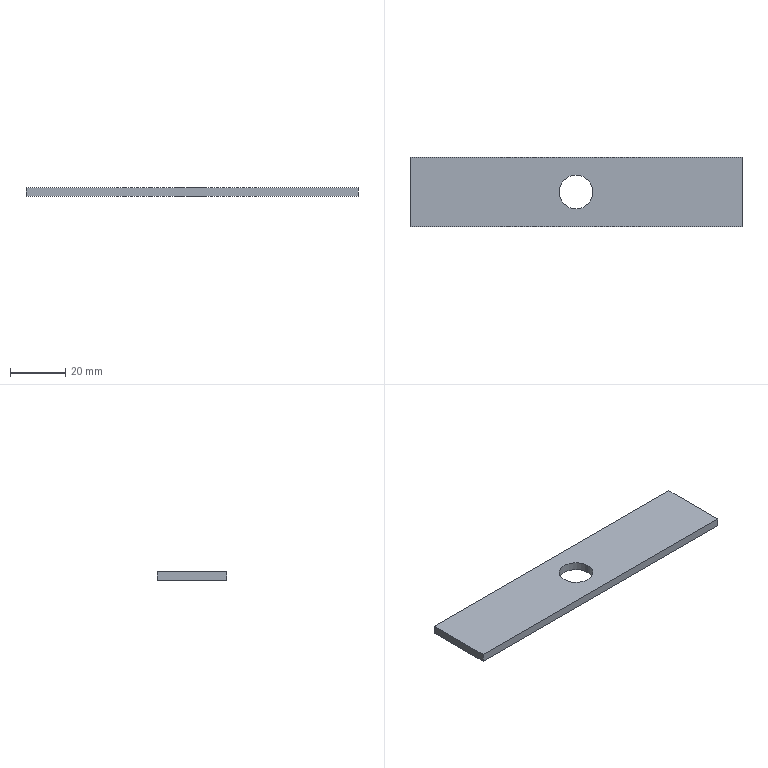Part | SolidWorks | features Extrusion 1, ICE 1 | 1 solid | 8 faces | box 120 x 25 x 3 mm | volume 8649 mm3 | plane 6 | cylinder 2 | commonest cylinder face diameters 12.2 x2
STEP:
#1=CARTESIAN_POINT('',(-6.1,0.,-1.5));
#2=VERTEX_POINT('',#1);
#3=CARTESIAN_POINT('',(6.1,0.,-1.5));
#4=VERTEX_POINT('',#3);
#5=CARTESIAN_POINT('',(0.,0.,-1.5));
#6=DIRECTION('',(0.,0.,1.));
#7=DIRECTION('',(1.,0.,0.));
#8=AXIS2_PLACEMENT_3D('',#5,#6,#7);
#9=CIRCLE('',#8,6.1);
#10=EDGE_CURVE('',#2,#4,#9,.T.);
#11=ORIENTED_EDGE('',*,*,#10,.F.);
#12=CARTESIAN_POINT('',(-6.1,0.,1.5));
#13=VERTEX_POINT('',#12);
#14=CARTESIAN_POINT('',(-6.1,0.,-11.5));
#15=DIRECTION('',(0.,0.,1.));
#16=VECTOR('',#15,1000.);
#17=LINE('',#14,#16);
#18=EDGE_CURVE('',#2,#13,#17,.T.);
#19=ORIENTED_EDGE('',*,*,#18,.T.);
#20=CARTESIAN_POINT('',(6.1,0.,1.5));
#21=VERTEX_POINT('',#20);
#22=CARTESIAN_POINT('',(0.,0.,1.5));
#23=DIRECTION('',(0.,0.,1.));
#24=DIRECTION('',(1.,0.,0.));
#25=AXIS2_PLACEMENT_3D('',#22,#23,#24);
#26=CIRCLE('',#25,6.1);
#27=EDGE_CURVE('',#13,#21,#26,.T.);
#28=ORIENTED_EDGE('',*,*,#27,.T.);
#29=CARTESIAN_POINT('',(6.1,0.,-11.5));
#30=DIRECTION('',(0.,0.,1.));
#31=VECTOR('',#30,1000.);
#32=LINE('',#29,#31);
#33=EDGE_CURVE('',#4,#21,#32,.T.);
#34=ORIENTED_EDGE('',*,*,#33,.F.);
#35=EDGE_LOOP('',(#11,#19,#28,#34));
#36=FACE_OUTER_BOUND('',#35,.T.);
#37=CARTESIAN_POINT('',(0.,0.,-11.5));
#38=DIRECTION('',(0.,0.,1.));
#39=DIRECTION('',(1.,0.,0.));
#40=AXIS2_PLACEMENT_3D('',#37,#38,#39);
#41=CYLINDRICAL_SURFACE('',#40,6.1);
#42=ADVANCED_FACE('',(#36),#41,.F.);
#43=CARTESIAN_POINT('',(-60.,12.5,1.5));
#44=VERTEX_POINT('',#43);
#45=CARTESIAN_POINT('',(-60.,-12.5,1.5));
#46=VERTEX_POINT('',#45);
#47=CARTESIAN_POINT('',(-60.,12.5,1.5));
#48=DIRECTION('',(0.,-1.,0.));
#49=VECTOR('',#48,1000.);
#50=LINE('',#47,#49);
#51=EDGE_CURVE('',#44,#46,#50,.T.);
#52=ORIENTED_EDGE('',*,*,#51,.F.);
#53=CARTESIAN_POINT('',(-60.,12.5,-1.5));
#54=VERTEX_POINT('',#53);
#55=CARTESIAN_POINT('',(-60.,12.5,-1.5));
#56=DIRECTION('',(0.,0.,1.));
#57=VECTOR('',#56,1000.);
#58=LINE('',#55,#57);
#59=EDGE_CURVE('',#54,#44,#58,.T.);
#60=ORIENTED_EDGE('',*,*,#59,.F.);
#61=CARTESIAN_POINT('',(-60.,-12.5,-1.5));
#62=VERTEX_POINT('',#61);
#63=CARTESIAN_POINT('',(-60.,12.5,-1.5));
#64=DIRECTION('',(0.,-1.,0.));
#65=VECTOR('',#64,1000.);
#66=LINE('',#63,#65);
#67=EDGE_CURVE('',#54,#62,#66,.T.);
#68=ORIENTED_EDGE('',*,*,#67,.T.);
#69=CARTESIAN_POINT('',(-60.,-12.5,-1.5));
#70=DIRECTION('',(0.,0.,1.));
#71=VECTOR('',#70,1000.);
#72=LINE('',#69,#71);
#73=EDGE_CURVE('',#62,#46,#72,.T.);
#74=ORIENTED_EDGE('',*,*,#73,.T.);
#75=EDGE_LOOP('',(#52,#60,#68,#74));
#76=FACE_OUTER_BOUND('',#75,.T.);
#77=CARTESIAN_POINT('',(-60.,12.5,-1.5));
#78=DIRECTION('',(-1.,0.,0.));
#79=DIRECTION('',(0.,0.,1.));
#80=AXIS2_PLACEMENT_3D('',#77,#78,#79);
#81=PLANE('',#80);
#82=ADVANCED_FACE('',(#76),#81,.T.);
#83=CARTESIAN_POINT('',(60.,12.5,1.5));
#84=VERTEX_POINT('',#83);
#85=CARTESIAN_POINT('',(60.,12.5,1.5));
#86=DIRECTION('',(-1.,0.,0.));
#87=VECTOR('',#86,1000.);
#88=LINE('',#85,#87);
#89=EDGE_CURVE('',#84,#44,#88,.T.);
#90=ORIENTED_EDGE('',*,*,#89,.F.);
#91=CARTESIAN_POINT('',(60.,12.5,-1.5));
#92=VERTEX_POINT('',#91);
#93=CARTESIAN_POINT('',(60.,12.5,-1.5));
#94=DIRECTION('',(0.,0.,1.));
#95=VECTOR('',#94,1000.);
#96=LINE('',#93,#95);
#97=EDGE_CURVE('',#92,#84,#96,.T.);
#98=ORIENTED_EDGE('',*,*,#97,.F.);
#99=CARTESIAN_POINT('',(60.,12.5,-1.5));
#100=DIRECTION('',(-1.,0.,0.));
#101=VECTOR('',#100,1000.);
#102=LINE('',#99,#101);
#103=EDGE_CURVE('',#92,#54,#102,.T.);
#104=ORIENTED_EDGE('',*,*,#103,.T.);
#105=ORIENTED_EDGE('',*,*,#59,.T.);
#106=EDGE_LOOP('',(#90,#98,#104,#105));
#107=FACE_OUTER_BOUND('',#106,.T.);
#108=CARTESIAN_POINT('',(60.,12.5,-1.5));
#109=DIRECTION('',(0.,1.,0.));
#110=DIRECTION('',(0.,0.,1.));
#111=AXIS2_PLACEMENT_3D('',#108,#109,#110);
#112=PLANE('',#111);
#113=ADVANCED_FACE('',(#107),#112,.T.);
#114=CARTESIAN_POINT('',(60.,-12.5,1.5));
#115=VERTEX_POINT('',#114);
#116=CARTESIAN_POINT('',(60.,-12.5,1.5));
#117=DIRECTION('',(0.,1.,0.));
#118=VECTOR('',#117,1000.);
#119=LINE('',#116,#118);
#120=EDGE_CURVE('',#115,#84,#119,.T.);
#121=ORIENTED_EDGE('',*,*,#120,.F.);
#122=CARTESIAN_POINT('',(60.,-12.5,-1.5));
#123=VERTEX_POINT('',#122);
#124=CARTESIAN_POINT('',(60.,-12.5,-1.5));
#125=DIRECTION('',(0.,0.,1.));
#126=VECTOR('',#125,1000.);
#127=LINE('',#124,#126);
#128=EDGE_CURVE('',#123,#115,#127,.T.);
#129=ORIENTED_EDGE('',*,*,#128,.F.);
#130=CARTESIAN_POINT('',(60.,-12.5,-1.5));
#131=DIRECTION('',(0.,1.,0.));
#132=VECTOR('',#131,1000.);
#133=LINE('',#130,#132);
#134=EDGE_CURVE('',#123,#92,#133,.T.);
#135=ORIENTED_EDGE('',*,*,#134,.T.);
#136=ORIENTED_EDGE('',*,*,#97,.T.);
#137=EDGE_LOOP('',(#121,#129,#135,#136));
#138=FACE_OUTER_BOUND('',#137,.T.);
#139=CARTESIAN_POINT('',(60.,-12.5,-1.5));
#140=DIRECTION('',(1.,0.,0.));
#141=DIRECTION('',(0.,0.,-1.));
#142=AXIS2_PLACEMENT_3D('',#139,#140,#141);
#143=PLANE('',#142);
#144=ADVANCED_FACE('',(#138),#143,.T.);
#145=CARTESIAN_POINT('',(-60.,-12.5,1.5));
#146=DIRECTION('',(1.,0.,0.));
#147=VECTOR('',#146,1000.);
#148=LINE('',#145,#147);
#149=EDGE_CURVE('',#46,#115,#148,.T.);
#150=ORIENTED_EDGE('',*,*,#149,.F.);
#151=ORIENTED_EDGE('',*,*,#73,.F.);
#152=CARTESIAN_POINT('',(-60.,-12.5,-1.5));
#153=DIRECTION('',(1.,0.,0.));
#154=VECTOR('',#153,1000.);
#155=LINE('',#152,#154);
#156=EDGE_CURVE('',#62,#123,#155,.T.);
#157=ORIENTED_EDGE('',*,*,#156,.T.);
#158=ORIENTED_EDGE('',*,*,#128,.T.);
#159=EDGE_LOOP('',(#150,#151,#157,#158));
#160=FACE_OUTER_BOUND('',#159,.T.);
#161=CARTESIAN_POINT('',(-60.,-12.5,-1.5));
#162=DIRECTION('',(0.,-1.,0.));
#163=DIRECTION('',(0.,0.,-1.));
#164=AXIS2_PLACEMENT_3D('',#161,#162,#163);
#165=PLANE('',#164);
#166=ADVANCED_FACE('',(#160),#165,.T.);
#167=CARTESIAN_POINT('',(0.,0.,-1.5));
#168=DIRECTION('',(0.,0.,1.));
#169=DIRECTION('',(1.,0.,0.));
#170=AXIS2_PLACEMENT_3D('',#167,#168,#169);
#171=CIRCLE('',#170,6.1);
#172=EDGE_CURVE('',#4,#2,#171,.T.);
#173=ORIENTED_EDGE('',*,*,#172,.T.);
#174=ORIENTED_EDGE('',*,*,#10,.T.);
#175=EDGE_LOOP('',(#173,#174));
#176=FACE_BOUND('',#175,.T.);
#177=ORIENTED_EDGE('',*,*,#67,.F.);
#178=ORIENTED_EDGE('',*,*,#103,.F.);
#179=ORIENTED_EDGE('',*,*,#134,.F.);
#180=ORIENTED_EDGE('',*,*,#156,.F.);
#181=EDGE_LOOP('',(#177,#178,#179,#180));
#182=FACE_OUTER_BOUND('',#181,.T.);
#183=CARTESIAN_POINT('',(0.,0.,-1.5));
#184=DIRECTION('',(0.,0.,1.));
#185=DIRECTION('',(1.,0.,0.));
#186=AXIS2_PLACEMENT_3D('',#183,#184,#185);
#187=PLANE('',#186);
#188=ADVANCED_FACE('',(#176,#182),#187,.F.);
#189=CARTESIAN_POINT('',(0.,0.,1.5));
#190=DIRECTION('',(0.,0.,1.));
#191=DIRECTION('',(1.,0.,0.));
#192=AXIS2_PLACEMENT_3D('',#189,#190,#191);
#193=CIRCLE('',#192,6.1);
#194=EDGE_CURVE('',#21,#13,#193,.T.);
#195=ORIENTED_EDGE('',*,*,#194,.F.);
#196=ORIENTED_EDGE('',*,*,#27,.F.);
#197=EDGE_LOOP('',(#195,#196));
#198=FACE_BOUND('',#197,.T.);
#199=ORIENTED_EDGE('',*,*,#51,.T.);
#200=ORIENTED_EDGE('',*,*,#149,.T.);
#201=ORIENTED_EDGE('',*,*,#120,.T.);
#202=ORIENTED_EDGE('',*,*,#89,.T.);
#203=EDGE_LOOP('',(#199,#200,#201,#202));
#204=FACE_OUTER_BOUND('',#203,.T.);
#205=CARTESIAN_POINT('',(0.,0.,1.5));
#206=DIRECTION('',(0.,0.,1.));
#207=DIRECTION('',(1.,0.,0.));
#208=AXIS2_PLACEMENT_3D('',#205,#206,#207);
#209=PLANE('',#208);
#210=ADVANCED_FACE('',(#198,#204),#209,.T.);
#211=ORIENTED_EDGE('',*,*,#18,.F.);
#212=ORIENTED_EDGE('',*,*,#172,.F.);
#213=ORIENTED_EDGE('',*,*,#33,.T.);
#214=ORIENTED_EDGE('',*,*,#194,.T.);
#215=EDGE_LOOP('',(#211,#212,#213,#214));
#216=FACE_OUTER_BOUND('',#215,.T.);
#217=CARTESIAN_POINT('',(0.,0.,-11.5));
#218=DIRECTION('',(0.,0.,1.));
#219=DIRECTION('',(1.,0.,0.));
#220=AXIS2_PLACEMENT_3D('',#217,#218,#219);
#221=CYLINDRICAL_SURFACE('',#220,6.1);
#222=ADVANCED_FACE('',(#216),#221,.F.);
#223=CLOSED_SHELL('',(#42,#82,#113,#144,#166,#188,#210,#222));
#224=MANIFOLD_SOLID_BREP('',#223);
#225=CARTESIAN_POINT('',(0.,0.,0.));
#226=DIRECTION('',(0.,0.,1.));
#227=DIRECTION('',(1.,0.,0.));
#228=AXIS2_PLACEMENT_3D('',#225,#226,#227);
#229=(LENGTH_UNIT()NAMED_UNIT(*)SI_UNIT(.MILLI.,.METRE.));
#230=UNCERTAINTY_MEASURE_WITH_UNIT(LENGTH_MEASURE(0.00001),#229,'','');
#231=(NAMED_UNIT(*)PLANE_ANGLE_UNIT()SI_UNIT($,.RADIAN.));
#232=(NAMED_UNIT(*)SI_UNIT($,.STERADIAN.)SOLID_ANGLE_UNIT());
#233=(GEOMETRIC_REPRESENTATION_CONTEXT(3)GLOBAL_UNCERTAINTY_ASSIGNED_CONTEXT((#230))GLOBAL_UNIT_ASSIGNED_CONTEXT((#229,#231,#232))REPRESENTATION_CONTEXT('',''));
#234=ADVANCED_BREP_SHAPE_REPRESENTATION('',(#224,#228),#233);